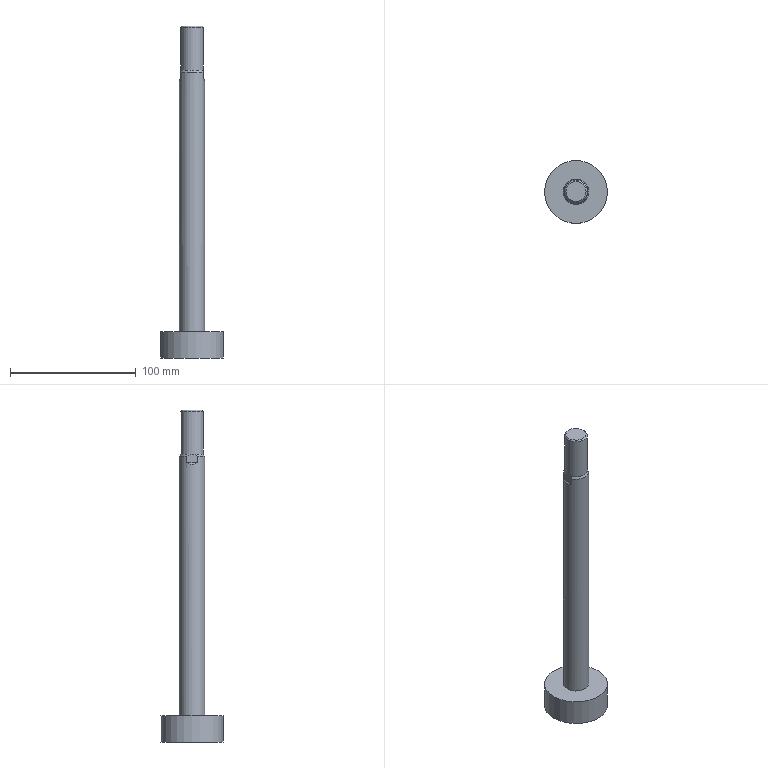Part | NX | features Hydraulic2.2_50 2 | 1 solid | 13 faces | box 50 x 50 x 263.5 mm | volume 115173 mm3 | plane 7 | cone 3 | cylinder 3 | commonest cylinder face diameters 18 x1 20 x1 50 x1
STEP:
#1=CARTESIAN_POINT('',(-8.,0.,263.5));
#2=VERTEX_POINT('',#1);
#3=CARTESIAN_POINT('',(0.,0.,263.5));
#4=DIRECTION('',(0.,0.,-1.));
#5=DIRECTION('',(-1.,0.,0.));
#6=AXIS2_PLACEMENT_3D('',#3,#4,#5);
#7=CIRCLE('',#6,8.);
#8=EDGE_CURVE('',#2,#2,#7,.T.);
#9=ORIENTED_EDGE('',*,*,#8,.F.);
#10=EDGE_LOOP('',(#9));
#11=FACE_BOUND('',#10,.T.);
#12=CARTESIAN_POINT('',(0.,0.,263.5));
#13=DIRECTION('',(0.,0.,1.));
#14=DIRECTION('',(1.,0.,0.));
#15=AXIS2_PLACEMENT_3D('',#12,#13,#14);
#16=PLANE('',#15);
#17=ADVANCED_FACE('',(#11),#16,.T.);
#18=ORIENTED_EDGE('',*,*,#8,.T.);
#19=EDGE_LOOP('',(#18));
#20=FACE_BOUND('',#19,.T.);
#21=CARTESIAN_POINT('',(9.,0.,262.5));
#22=VERTEX_POINT('',#21);
#23=CARTESIAN_POINT('',(0.,0.,262.5));
#24=DIRECTION('',(0.,0.,1.));
#25=DIRECTION('',(1.,0.,0.));
#26=AXIS2_PLACEMENT_3D('',#23,#24,#25);
#27=CIRCLE('',#26,9.);
#28=EDGE_CURVE('',#22,#22,#27,.F.);
#29=ORIENTED_EDGE('',*,*,#28,.F.);
#30=EDGE_LOOP('',(#29));
#31=FACE_BOUND('',#30,.T.);
#32=CARTESIAN_POINT('',(0.,0.,262.5));
#33=DIRECTION('',(0.,0.,-1.));
#34=DIRECTION('',(-1.,0.,0.));
#35=AXIS2_PLACEMENT_3D('',#32,#33,#34);
#36=CONICAL_SURFACE('',#35,9.,0.7854);
#37=ADVANCED_FACE('',(#20,#31),#36,.T.);
#38=CARTESIAN_POINT('',(-25.,0.,0.));
#39=VERTEX_POINT('',#38);
#40=CARTESIAN_POINT('',(0.,0.,0.));
#41=DIRECTION('',(0.,0.,-1.));
#42=DIRECTION('',(-1.,0.,0.));
#43=AXIS2_PLACEMENT_3D('',#40,#41,#42);
#44=CIRCLE('',#43,25.);
#45=EDGE_CURVE('',#39,#39,#44,.F.);
#46=ORIENTED_EDGE('',*,*,#45,.F.);
#47=EDGE_LOOP('',(#46));
#48=FACE_BOUND('',#47,.T.);
#49=CARTESIAN_POINT('',(0.,0.,0.));
#50=DIRECTION('',(0.,0.,1.));
#51=DIRECTION('',(1.,0.,0.));
#52=AXIS2_PLACEMENT_3D('',#49,#50,#51);
#53=PLANE('',#52);
#54=ADVANCED_FACE('',(#48),#53,.F.);
#55=CARTESIAN_POINT('',(-9.,0.,228.5));
#56=VERTEX_POINT('',#55);
#57=CARTESIAN_POINT('',(9.,0.,228.5));
#58=VERTEX_POINT('',#57);
#59=CARTESIAN_POINT('',(0.,0.,228.5));
#60=DIRECTION('',(0.,0.,-1.));
#61=DIRECTION('',(-1.,0.,0.));
#62=AXIS2_PLACEMENT_3D('',#59,#60,#61);
#63=CIRCLE('',#62,9.);
#64=EDGE_CURVE('',#56,#58,#63,.T.);
#65=ORIENTED_EDGE('',*,*,#64,.F.);
#66=CARTESIAN_POINT('',(0.,0.,228.5));
#67=DIRECTION('',(0.,0.,-1.));
#68=DIRECTION('',(-1.,0.,0.));
#69=AXIS2_PLACEMENT_3D('',#66,#67,#68);
#70=CIRCLE('',#69,9.);
#71=EDGE_CURVE('',#58,#56,#70,.T.);
#72=ORIENTED_EDGE('',*,*,#71,.F.);
#73=EDGE_LOOP('',(#65,#72));
#74=FACE_BOUND('',#73,.T.);
#75=ORIENTED_EDGE('',*,*,#28,.T.);
#76=EDGE_LOOP('',(#75));
#77=FACE_BOUND('',#76,.T.);
#78=CARTESIAN_POINT('',(0.,0.,101.998));
#79=DIRECTION('',(0.,0.,1.));
#80=DIRECTION('',(1.,0.,0.));
#81=AXIS2_PLACEMENT_3D('',#78,#79,#80);
#82=CYLINDRICAL_SURFACE('',#81,9.);
#83=ADVANCED_FACE('',(#74,#77),#82,.T.);
#84=CARTESIAN_POINT('',(-9.,4.359,226.768));
#85=VERTEX_POINT('',#84);
#86=CARTESIAN_POINT('',(-9.,4.359,226.768));
#87=CARTESIAN_POINT('',(-9.,3.084,227.731));
#88=CARTESIAN_POINT('',(-9.,1.617,228.5));
#89=CARTESIAN_POINT('',(-9.,0.,228.5));
#90=B_SPLINE_CURVE_WITH_KNOTS('',3,(#86,#87,#88,#89),.UNSPECIFIED.,.F.,.F.,(4,4),(0.,0.004725),.UNSPECIFIED.);
#91=EDGE_CURVE('',#85,#56,#90,.T.);
#92=ORIENTED_EDGE('',*,*,#91,.T.);
#93=ORIENTED_EDGE('',*,*,#64,.T.);
#94=CARTESIAN_POINT('',(9.,4.359,226.768));
#95=VERTEX_POINT('',#94);
#96=CARTESIAN_POINT('',(9.,0.,228.5));
#97=CARTESIAN_POINT('',(9.,1.612,228.5));
#98=CARTESIAN_POINT('',(9.,3.083,227.732));
#99=CARTESIAN_POINT('',(9.,4.359,226.768));
#100=B_SPLINE_CURVE_WITH_KNOTS('',3,(#96,#97,#98,#99),.UNSPECIFIED.,.F.,.F.,(4,4),(0.,0.004745),.UNSPECIFIED.);
#101=EDGE_CURVE('',#58,#95,#100,.T.);
#102=ORIENTED_EDGE('',*,*,#101,.T.);
#103=CARTESIAN_POINT('',(0.,0.,226.768));
#104=DIRECTION('',(0.,0.,-1.));
#105=DIRECTION('',(-1.,0.,0.));
#106=AXIS2_PLACEMENT_3D('',#103,#104,#105);
#107=CIRCLE('',#106,10.);
#108=EDGE_CURVE('',#85,#95,#107,.T.);
#109=ORIENTED_EDGE('',*,*,#108,.F.);
#110=EDGE_LOOP('',(#92,#93,#102,#109));
#111=FACE_BOUND('',#110,.T.);
#112=CARTESIAN_POINT('',(0.,0.,226.768));
#113=DIRECTION('',(0.,0.,-1.));
#114=DIRECTION('',(0.,1.,0.));
#115=AXIS2_PLACEMENT_3D('',#112,#113,#114);
#116=CONICAL_SURFACE('',#115,10.,0.5236);
#117=ADVANCED_FACE('',(#111),#116,.T.);
#118=ORIENTED_EDGE('',*,*,#45,.T.);
#119=EDGE_LOOP('',(#118));
#120=FACE_BOUND('',#119,.T.);
#121=CARTESIAN_POINT('',(-25.,0.,21.));
#122=VERTEX_POINT('',#121);
#123=CARTESIAN_POINT('',(0.,0.,21.));
#124=DIRECTION('',(0.,0.,-1.));
#125=DIRECTION('',(-1.,0.,0.));
#126=AXIS2_PLACEMENT_3D('',#123,#124,#125);
#127=CIRCLE('',#126,25.);
#128=EDGE_CURVE('',#122,#122,#127,.F.);
#129=ORIENTED_EDGE('',*,*,#128,.F.);
#130=EDGE_LOOP('',(#129));
#131=FACE_BOUND('',#130,.T.);
#132=CARTESIAN_POINT('',(0.,0.,21.));
#133=DIRECTION('',(0.,0.,-1.));
#134=DIRECTION('',(-1.,0.,0.));
#135=AXIS2_PLACEMENT_3D('',#132,#133,#134);
#136=CYLINDRICAL_SURFACE('',#135,25.);
#137=ADVANCED_FACE('',(#120,#131),#136,.T.);
#138=CARTESIAN_POINT('',(9.,4.359,221.5));
#139=VERTEX_POINT('',#138);
#140=CARTESIAN_POINT('',(9.,-4.359,221.5));
#141=VERTEX_POINT('',#140);
#142=CARTESIAN_POINT('',(9.,-25.,221.5));
#143=DIRECTION('',(0.,1.,0.));
#144=VECTOR('',#143,1000.);
#145=LINE('',#142,#144);
#146=EDGE_CURVE('',#139,#141,#145,.F.);
#147=ORIENTED_EDGE('',*,*,#146,.T.);
#148=CARTESIAN_POINT('',(0.,0.,230.5));
#149=DIRECTION('',(-0.7071,0.,-0.7071));
#150=DIRECTION('',(0.7071,0.,-0.7071));
#151=AXIS2_PLACEMENT_3D('',#148,#149,#150);
#152=ELLIPSE('',#151,14.142,10.);
#153=EDGE_CURVE('',#139,#141,#152,.T.);
#154=ORIENTED_EDGE('',*,*,#153,.F.);
#155=EDGE_LOOP('',(#147,#154));
#156=FACE_BOUND('',#155,.T.);
#157=CARTESIAN_POINT('',(9.,-25.,221.5));
#158=DIRECTION('',(-0.7071,0.,-0.7071));
#159=DIRECTION('',(-0.7071,0.,0.7071));
#160=AXIS2_PLACEMENT_3D('',#157,#158,#159);
#161=PLANE('',#160);
#162=ADVANCED_FACE('',(#156),#161,.F.);
#163=CARTESIAN_POINT('',(9.,-4.359,226.768));
#164=VERTEX_POINT('',#163);
#165=CARTESIAN_POINT('',(9.,-4.359,226.768));
#166=CARTESIAN_POINT('',(9.,-3.084,227.731));
#167=CARTESIAN_POINT('',(9.,-1.617,228.5));
#168=CARTESIAN_POINT('',(9.,0.,228.5));
#169=B_SPLINE_CURVE_WITH_KNOTS('',3,(#165,#166,#167,#168),.UNSPECIFIED.,.F.,.F.,(4,4),(0.,0.004725),.UNSPECIFIED.);
#170=EDGE_CURVE('',#164,#58,#169,.T.);
#171=ORIENTED_EDGE('',*,*,#170,.F.);
#172=CARTESIAN_POINT('',(9.,-4.359,291.784));
#173=DIRECTION('',(0.,0.,-1.));
#174=VECTOR('',#173,1000.);
#175=LINE('',#172,#174);
#176=EDGE_CURVE('',#141,#164,#175,.F.);
#177=ORIENTED_EDGE('',*,*,#176,.F.);
#178=ORIENTED_EDGE('',*,*,#146,.F.);
#179=CARTESIAN_POINT('',(9.,4.359,291.784));
#180=DIRECTION('',(0.,0.,-1.));
#181=VECTOR('',#180,1000.);
#182=LINE('',#179,#181);
#183=EDGE_CURVE('',#95,#139,#182,.T.);
#184=ORIENTED_EDGE('',*,*,#183,.F.);
#185=ORIENTED_EDGE('',*,*,#101,.F.);
#186=EDGE_LOOP('',(#171,#177,#178,#184,#185));
#187=FACE_BOUND('',#186,.T.);
#188=CARTESIAN_POINT('',(9.,-25.,228.5));
#189=DIRECTION('',(-1.,0.,0.));
#190=DIRECTION('',(0.,0.,1.));
#191=AXIS2_PLACEMENT_3D('',#188,#189,#190);
#192=PLANE('',#191);
#193=ADVANCED_FACE('',(#187),#192,.F.);
#194=CARTESIAN_POINT('',(-9.,-4.359,226.768));
#195=VERTEX_POINT('',#194);
#196=CARTESIAN_POINT('',(-9.,0.,228.5));
#197=CARTESIAN_POINT('',(-9.,-1.612,228.5));
#198=CARTESIAN_POINT('',(-9.,-3.083,227.732));
#199=CARTESIAN_POINT('',(-9.,-4.359,226.768));
#200=B_SPLINE_CURVE_WITH_KNOTS('',3,(#196,#197,#198,#199),.UNSPECIFIED.,.F.,.F.,(4,4),(0.,0.004745),.UNSPECIFIED.);
#201=EDGE_CURVE('',#56,#195,#200,.T.);
#202=ORIENTED_EDGE('',*,*,#201,.T.);
#203=CARTESIAN_POINT('',(0.,0.,226.768));
#204=DIRECTION('',(0.,0.,-1.));
#205=DIRECTION('',(-1.,0.,0.));
#206=AXIS2_PLACEMENT_3D('',#203,#204,#205);
#207=CIRCLE('',#206,10.);
#208=EDGE_CURVE('',#164,#195,#207,.T.);
#209=ORIENTED_EDGE('',*,*,#208,.F.);
#210=ORIENTED_EDGE('',*,*,#170,.T.);
#211=ORIENTED_EDGE('',*,*,#71,.T.);
#212=EDGE_LOOP('',(#202,#209,#210,#211));
#213=FACE_BOUND('',#212,.T.);
#214=CARTESIAN_POINT('',(0.,0.,226.768));
#215=DIRECTION('',(0.,0.,-1.));
#216=DIRECTION('',(0.,1.,0.));
#217=AXIS2_PLACEMENT_3D('',#214,#215,#216);
#218=CONICAL_SURFACE('',#217,10.,0.5236);
#219=ADVANCED_FACE('',(#213),#218,.T.);
#220=ORIENTED_EDGE('',*,*,#91,.F.);
#221=CARTESIAN_POINT('',(-9.,4.359,221.5));
#222=VERTEX_POINT('',#221);
#223=CARTESIAN_POINT('',(-9.,4.359,291.784));
#224=DIRECTION('',(0.,0.,-1.));
#225=VECTOR('',#224,1000.);
#226=LINE('',#223,#225);
#227=EDGE_CURVE('',#222,#85,#226,.F.);
#228=ORIENTED_EDGE('',*,*,#227,.F.);
#229=CARTESIAN_POINT('',(-9.,-4.359,221.5));
#230=VERTEX_POINT('',#229);
#231=CARTESIAN_POINT('',(-9.,-25.,221.5));
#232=DIRECTION('',(0.,1.,0.));
#233=VECTOR('',#232,1000.);
#234=LINE('',#231,#233);
#235=EDGE_CURVE('',#222,#230,#234,.F.);
#236=ORIENTED_EDGE('',*,*,#235,.T.);
#237=CARTESIAN_POINT('',(-9.,-4.359,291.784));
#238=DIRECTION('',(0.,0.,-1.));
#239=VECTOR('',#238,1000.);
#240=LINE('',#237,#239);
#241=EDGE_CURVE('',#195,#230,#240,.T.);
#242=ORIENTED_EDGE('',*,*,#241,.F.);
#243=ORIENTED_EDGE('',*,*,#201,.F.);
#244=EDGE_LOOP('',(#220,#228,#236,#242,#243));
#245=FACE_BOUND('',#244,.T.);
#246=CARTESIAN_POINT('',(-9.,-25.,228.5));
#247=DIRECTION('',(1.,0.,0.));
#248=DIRECTION('',(0.,0.,-1.));
#249=AXIS2_PLACEMENT_3D('',#246,#247,#248);
#250=PLANE('',#249);
#251=ADVANCED_FACE('',(#245),#250,.F.);
#252=ORIENTED_EDGE('',*,*,#235,.F.);
#253=CARTESIAN_POINT('',(0.,0.,230.5));
#254=DIRECTION('',(0.7071,0.,-0.7071));
#255=DIRECTION('',(-0.7071,0.,-0.7071));
#256=AXIS2_PLACEMENT_3D('',#253,#254,#255);
#257=ELLIPSE('',#256,14.142,10.);
#258=EDGE_CURVE('',#230,#222,#257,.T.);
#259=ORIENTED_EDGE('',*,*,#258,.F.);
#260=EDGE_LOOP('',(#252,#259));
#261=FACE_BOUND('',#260,.T.);
#262=CARTESIAN_POINT('',(-9.,-25.,221.5));
#263=DIRECTION('',(0.7071,0.,-0.7071));
#264=DIRECTION('',(-0.7071,0.,-0.7071));
#265=AXIS2_PLACEMENT_3D('',#262,#263,#264);
#266=PLANE('',#265);
#267=ADVANCED_FACE('',(#261),#266,.F.);
#268=CARTESIAN_POINT('',(-10.,0.,21.));
#269=VERTEX_POINT('',#268);
#270=CARTESIAN_POINT('',(0.,0.,21.));
#271=DIRECTION('',(0.,0.,-1.));
#272=DIRECTION('',(-1.,0.,0.));
#273=AXIS2_PLACEMENT_3D('',#270,#271,#272);
#274=CIRCLE('',#273,10.);
#275=EDGE_CURVE('',#269,#269,#274,.F.);
#276=ORIENTED_EDGE('',*,*,#275,.F.);
#277=EDGE_LOOP('',(#276));
#278=FACE_BOUND('',#277,.T.);
#279=ORIENTED_EDGE('',*,*,#128,.T.);
#280=EDGE_LOOP('',(#279));
#281=FACE_BOUND('',#280,.T.);
#282=CARTESIAN_POINT('',(0.,0.,21.));
#283=DIRECTION('',(0.,0.,1.));
#284=DIRECTION('',(1.,0.,0.));
#285=AXIS2_PLACEMENT_3D('',#282,#283,#284);
#286=PLANE('',#285);
#287=ADVANCED_FACE('',(#278,#281),#286,.T.);
#288=ORIENTED_EDGE('',*,*,#183,.T.);
#289=ORIENTED_EDGE('',*,*,#153,.T.);
#290=ORIENTED_EDGE('',*,*,#176,.T.);
#291=ORIENTED_EDGE('',*,*,#208,.T.);
#292=ORIENTED_EDGE('',*,*,#241,.T.);
#293=ORIENTED_EDGE('',*,*,#258,.T.);
#294=ORIENTED_EDGE('',*,*,#227,.T.);
#295=ORIENTED_EDGE('',*,*,#108,.T.);
#296=EDGE_LOOP('',(#288,#289,#290,#291,#292,#293,#294,#295));
#297=FACE_BOUND('',#296,.T.);
#298=ORIENTED_EDGE('',*,*,#275,.T.);
#299=EDGE_LOOP('',(#298));
#300=FACE_BOUND('',#299,.T.);
#301=CARTESIAN_POINT('',(0.,0.,291.784));
#302=DIRECTION('',(0.,0.,-1.));
#303=DIRECTION('',(-1.,0.,0.));
#304=AXIS2_PLACEMENT_3D('',#301,#302,#303);
#305=CYLINDRICAL_SURFACE('',#304,10.);
#306=ADVANCED_FACE('',(#297,#300),#305,.T.);
#307=CLOSED_SHELL('',(#17,#37,#54,#83,#117,#137,#162,#193,#219,#251,#267,#287,#306));
#308=MANIFOLD_SOLID_BREP('',#307);
#309=(LENGTH_UNIT()NAMED_UNIT(*)SI_UNIT(.MILLI.,.METRE.));
#310=UNCERTAINTY_MEASURE_WITH_UNIT(LENGTH_MEASURE(0.0508),#309,'','');
#311=(NAMED_UNIT(*)PLANE_ANGLE_UNIT()SI_UNIT($,.RADIAN.));
#312=(NAMED_UNIT(*)SI_UNIT($,.STERADIAN.)SOLID_ANGLE_UNIT());
#313=(GEOMETRIC_REPRESENTATION_CONTEXT(3)GLOBAL_UNCERTAINTY_ASSIGNED_CONTEXT((#310))GLOBAL_UNIT_ASSIGNED_CONTEXT((#309,#311,#312))REPRESENTATION_CONTEXT('',''));
#314=ADVANCED_BREP_SHAPE_REPRESENTATION('',(#308),#313);